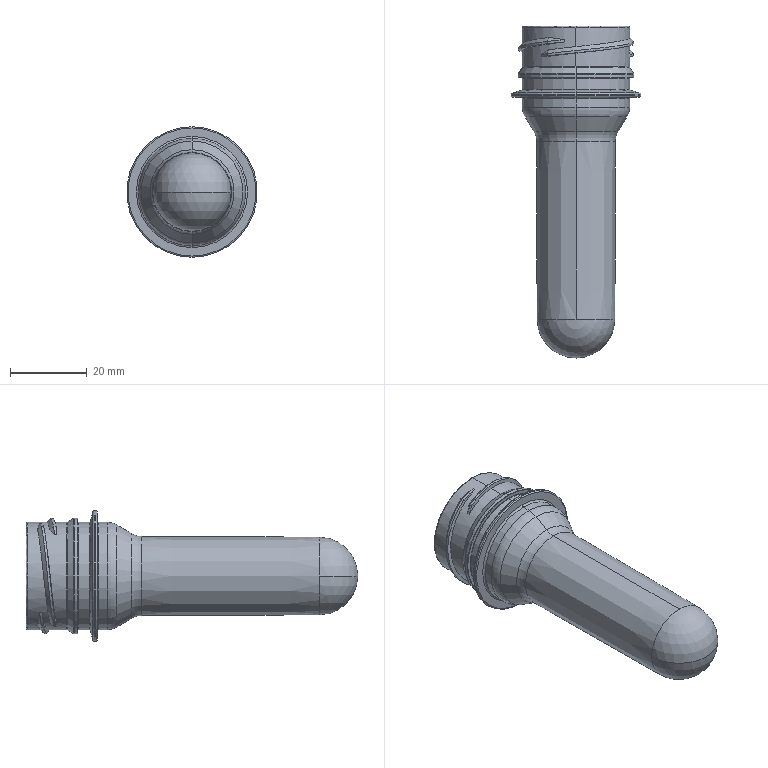Part | STEP file | 30-25 bottle preform_default | 1 solid | 88 faces | box 34 x 86.5 x 34 mm | volume 12147 mm3 | spline 29 | torus 28 | cone 14 | cylinder 10 | sphere 4 | plane 3 | commonest cylinder face diameters 28 x6 30.2 x2 34 x2